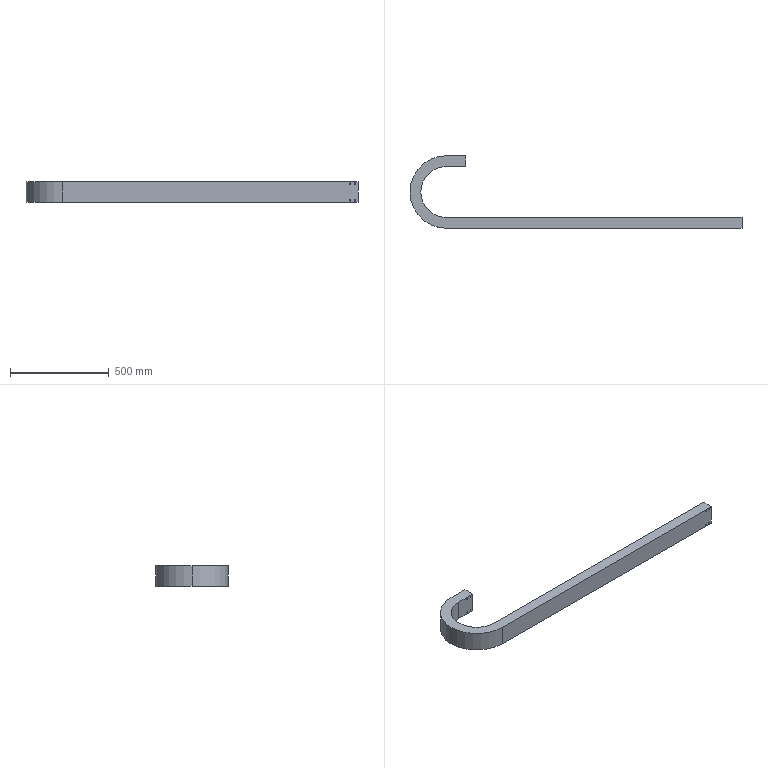Part | NX | features BREP 1 | 1 solid | 40 faces | box 1684 x 368 x 102 mm | volume 6232156 mm3 | cylinder 22 | plane 18 | commonest cylinder face diameters 5.5 x8 6 x8 258 x2 368 x2 278 x1 348 x1
STEP:
#1=CARTESIAN_POINT('',(1460.2,-184.,5.25));
#2=VERTEX_POINT('',#1);
#3=CARTESIAN_POINT('',(1460.2,-184.,11.25));
#4=VERTEX_POINT('',#3);
#5=CARTESIAN_POINT('',(1460.2,-184.,8.25));
#6=DIRECTION('',(0.,1.,0.));
#7=DIRECTION('',(0.,0.,1.));
#8=AXIS2_PLACEMENT_3D('',#5,#6,#7);
#9=CIRCLE('',#8,3.);
#10=EDGE_CURVE('',#2,#4,#9,.T.);
#11=ORIENTED_EDGE('',*,*,#10,.F.);
#12=CARTESIAN_POINT('',(1460.2,-129.,5.25));
#13=VERTEX_POINT('',#12);
#14=CARTESIAN_POINT('',(1460.2,-231.,5.25));
#15=DIRECTION('',(0.,1.,0.));
#16=VECTOR('',#15,1000.);
#17=LINE('',#14,#16);
#18=EDGE_CURVE('',#13,#2,#17,.F.);
#19=ORIENTED_EDGE('',*,*,#18,.F.);
#20=CARTESIAN_POINT('',(1460.2,-129.,11.25));
#21=VERTEX_POINT('',#20);
#22=CARTESIAN_POINT('',(1460.2,-129.,8.25));
#23=DIRECTION('',(0.,1.,0.));
#24=DIRECTION('',(0.,0.,1.));
#25=AXIS2_PLACEMENT_3D('',#22,#23,#24);
#26=CIRCLE('',#25,3.);
#27=EDGE_CURVE('',#13,#21,#26,.T.);
#28=ORIENTED_EDGE('',*,*,#27,.T.);
#29=CARTESIAN_POINT('',(1460.2,-231.,11.25));
#30=DIRECTION('',(0.,1.,0.));
#31=VECTOR('',#30,1000.);
#32=LINE('',#29,#31);
#33=EDGE_CURVE('',#21,#4,#32,.F.);
#34=ORIENTED_EDGE('',*,*,#33,.T.);
#35=EDGE_LOOP('',(#11,#19,#28,#34));
#36=FACE_BOUND('',#35,.T.);
#37=CARTESIAN_POINT('',(1460.2,-231.,8.25));
#38=DIRECTION('',(0.,1.,0.));
#39=DIRECTION('',(0.,0.,1.));
#40=AXIS2_PLACEMENT_3D('',#37,#38,#39);
#41=CYLINDRICAL_SURFACE('',#40,3.);
#42=ADVANCED_FACE('',(#36),#41,.F.);
#43=CARTESIAN_POINT('',(1484.35,-184.,90.75));
#44=VERTEX_POINT('',#43);
#45=CARTESIAN_POINT('',(1484.35,-184.,96.75));
#46=VERTEX_POINT('',#45);
#47=CARTESIAN_POINT('',(1484.35,-184.,93.75));
#48=DIRECTION('',(0.,1.,0.));
#49=DIRECTION('',(0.,0.,1.));
#50=AXIS2_PLACEMENT_3D('',#47,#48,#49);
#51=CIRCLE('',#50,3.);
#52=EDGE_CURVE('',#44,#46,#51,.T.);
#53=ORIENTED_EDGE('',*,*,#52,.F.);
#54=CARTESIAN_POINT('',(1484.35,-129.,90.75));
#55=VERTEX_POINT('',#54);
#56=CARTESIAN_POINT('',(1484.35,-231.,90.75));
#57=DIRECTION('',(0.,1.,0.));
#58=VECTOR('',#57,1000.);
#59=LINE('',#56,#58);
#60=EDGE_CURVE('',#55,#44,#59,.F.);
#61=ORIENTED_EDGE('',*,*,#60,.F.);
#62=CARTESIAN_POINT('',(1484.35,-129.,96.75));
#63=VERTEX_POINT('',#62);
#64=CARTESIAN_POINT('',(1484.35,-129.,93.75));
#65=DIRECTION('',(0.,1.,0.));
#66=DIRECTION('',(0.,0.,1.));
#67=AXIS2_PLACEMENT_3D('',#64,#65,#66);
#68=CIRCLE('',#67,3.);
#69=EDGE_CURVE('',#55,#63,#68,.T.);
#70=ORIENTED_EDGE('',*,*,#69,.T.);
#71=CARTESIAN_POINT('',(1484.35,-231.,96.75));
#72=DIRECTION('',(0.,1.,0.));
#73=VECTOR('',#72,1000.);
#74=LINE('',#71,#73);
#75=EDGE_CURVE('',#63,#46,#74,.F.);
#76=ORIENTED_EDGE('',*,*,#75,.T.);
#77=EDGE_LOOP('',(#53,#61,#70,#76));
#78=FACE_BOUND('',#77,.T.);
#79=CARTESIAN_POINT('',(1484.35,-231.,93.75));
#80=DIRECTION('',(0.,1.,0.));
#81=DIRECTION('',(0.,0.,1.));
#82=AXIS2_PLACEMENT_3D('',#79,#80,#81);
#83=CYLINDRICAL_SURFACE('',#82,3.);
#84=ADVANCED_FACE('',(#78),#83,.F.);
#85=CARTESIAN_POINT('',(1460.2,-184.,90.75));
#86=VERTEX_POINT('',#85);
#87=CARTESIAN_POINT('',(1460.2,-184.,96.75));
#88=VERTEX_POINT('',#87);
#89=CARTESIAN_POINT('',(1460.2,-184.,93.75));
#90=DIRECTION('',(0.,1.,0.));
#91=DIRECTION('',(0.,0.,1.));
#92=AXIS2_PLACEMENT_3D('',#89,#90,#91);
#93=CIRCLE('',#92,3.);
#94=EDGE_CURVE('',#86,#88,#93,.T.);
#95=ORIENTED_EDGE('',*,*,#94,.F.);
#96=CARTESIAN_POINT('',(1460.2,-129.,90.75));
#97=VERTEX_POINT('',#96);
#98=CARTESIAN_POINT('',(1460.2,-231.,90.75));
#99=DIRECTION('',(0.,1.,0.));
#100=VECTOR('',#99,1000.);
#101=LINE('',#98,#100);
#102=EDGE_CURVE('',#97,#86,#101,.F.);
#103=ORIENTED_EDGE('',*,*,#102,.F.);
#104=CARTESIAN_POINT('',(1460.2,-129.,96.75));
#105=VERTEX_POINT('',#104);
#106=CARTESIAN_POINT('',(1460.2,-129.,93.75));
#107=DIRECTION('',(0.,1.,0.));
#108=DIRECTION('',(0.,0.,1.));
#109=AXIS2_PLACEMENT_3D('',#106,#107,#108);
#110=CIRCLE('',#109,3.);
#111=EDGE_CURVE('',#97,#105,#110,.T.);
#112=ORIENTED_EDGE('',*,*,#111,.T.);
#113=CARTESIAN_POINT('',(1460.2,-231.,96.75));
#114=DIRECTION('',(0.,1.,0.));
#115=VECTOR('',#114,1000.);
#116=LINE('',#113,#115);
#117=EDGE_CURVE('',#105,#88,#116,.F.);
#118=ORIENTED_EDGE('',*,*,#117,.T.);
#119=EDGE_LOOP('',(#95,#103,#112,#118));
#120=FACE_BOUND('',#119,.T.);
#121=CARTESIAN_POINT('',(1460.2,-231.,93.75));
#122=DIRECTION('',(0.,1.,0.));
#123=DIRECTION('',(0.,0.,1.));
#124=AXIS2_PLACEMENT_3D('',#121,#122,#123);
#125=CYLINDRICAL_SURFACE('',#124,3.);
#126=ADVANCED_FACE('',(#120),#125,.F.);
#127=CARTESIAN_POINT('',(1484.35,-184.,5.25));
#128=VERTEX_POINT('',#127);
#129=CARTESIAN_POINT('',(1484.35,-184.,11.25));
#130=VERTEX_POINT('',#129);
#131=CARTESIAN_POINT('',(1484.35,-184.,8.25));
#132=DIRECTION('',(0.,1.,0.));
#133=DIRECTION('',(0.,0.,1.));
#134=AXIS2_PLACEMENT_3D('',#131,#132,#133);
#135=CIRCLE('',#134,3.);
#136=EDGE_CURVE('',#128,#130,#135,.T.);
#137=ORIENTED_EDGE('',*,*,#136,.F.);
#138=CARTESIAN_POINT('',(1484.35,-129.,5.25));
#139=VERTEX_POINT('',#138);
#140=CARTESIAN_POINT('',(1484.35,-231.,5.25));
#141=DIRECTION('',(0.,1.,0.));
#142=VECTOR('',#141,1000.);
#143=LINE('',#140,#142);
#144=EDGE_CURVE('',#139,#128,#143,.F.);
#145=ORIENTED_EDGE('',*,*,#144,.F.);
#146=CARTESIAN_POINT('',(1484.35,-129.,11.25));
#147=VERTEX_POINT('',#146);
#148=CARTESIAN_POINT('',(1484.35,-129.,8.25));
#149=DIRECTION('',(0.,1.,0.));
#150=DIRECTION('',(0.,0.,1.));
#151=AXIS2_PLACEMENT_3D('',#148,#149,#150);
#152=CIRCLE('',#151,3.);
#153=EDGE_CURVE('',#139,#147,#152,.T.);
#154=ORIENTED_EDGE('',*,*,#153,.T.);
#155=CARTESIAN_POINT('',(1484.35,-231.,11.25));
#156=DIRECTION('',(0.,1.,0.));
#157=VECTOR('',#156,1000.);
#158=LINE('',#155,#157);
#159=EDGE_CURVE('',#147,#130,#158,.F.);
#160=ORIENTED_EDGE('',*,*,#159,.T.);
#161=EDGE_LOOP('',(#137,#145,#154,#160));
#162=FACE_BOUND('',#161,.T.);
#163=CARTESIAN_POINT('',(1484.35,-231.,8.25));
#164=DIRECTION('',(0.,1.,0.));
#165=DIRECTION('',(0.,0.,1.));
#166=AXIS2_PLACEMENT_3D('',#163,#164,#165);
#167=CYLINDRICAL_SURFACE('',#166,3.);
#168=ADVANCED_FACE('',(#162),#167,.F.);
#169=CARTESIAN_POINT('',(84.35,129.,5.5));
#170=VERTEX_POINT('',#169);
#171=CARTESIAN_POINT('',(84.35,129.,11.));
#172=VERTEX_POINT('',#171);
#173=CARTESIAN_POINT('',(84.35,129.,8.25));
#174=DIRECTION('',(0.,1.,0.));
#175=DIRECTION('',(0.,0.,1.));
#176=AXIS2_PLACEMENT_3D('',#173,#174,#175);
#177=CIRCLE('',#176,2.75);
#178=EDGE_CURVE('',#170,#172,#177,.T.);
#179=ORIENTED_EDGE('',*,*,#178,.F.);
#180=CARTESIAN_POINT('',(84.35,184.,5.5));
#181=VERTEX_POINT('',#180);
#182=CARTESIAN_POINT('',(84.35,184.,5.5));
#183=DIRECTION('',(0.,1.,0.));
#184=VECTOR('',#183,1000.);
#185=LINE('',#182,#184);
#186=EDGE_CURVE('',#181,#170,#185,.F.);
#187=ORIENTED_EDGE('',*,*,#186,.F.);
#188=CARTESIAN_POINT('',(84.35,184.,11.));
#189=VERTEX_POINT('',#188);
#190=CARTESIAN_POINT('',(84.35,184.,8.25));
#191=DIRECTION('',(0.,1.,0.));
#192=DIRECTION('',(0.,0.,1.));
#193=AXIS2_PLACEMENT_3D('',#190,#191,#192);
#194=CIRCLE('',#193,2.75);
#195=EDGE_CURVE('',#181,#189,#194,.T.);
#196=ORIENTED_EDGE('',*,*,#195,.T.);
#197=CARTESIAN_POINT('',(84.35,184.,11.));
#198=DIRECTION('',(0.,1.,0.));
#199=VECTOR('',#198,1000.);
#200=LINE('',#197,#199);
#201=EDGE_CURVE('',#189,#172,#200,.F.);
#202=ORIENTED_EDGE('',*,*,#201,.T.);
#203=EDGE_LOOP('',(#179,#187,#196,#202));
#204=FACE_BOUND('',#203,.T.);
#205=CARTESIAN_POINT('',(84.35,184.,8.25));
#206=DIRECTION('',(0.,1.,0.));
#207=DIRECTION('',(0.,0.,1.));
#208=AXIS2_PLACEMENT_3D('',#205,#206,#207);
#209=CYLINDRICAL_SURFACE('',#208,2.75);
#210=ADVANCED_FACE('',(#204),#209,.F.);
#211=CARTESIAN_POINT('',(60.2,129.,5.5));
#212=VERTEX_POINT('',#211);
#213=CARTESIAN_POINT('',(60.2,129.,11.));
#214=VERTEX_POINT('',#213);
#215=CARTESIAN_POINT('',(60.2,129.,8.25));
#216=DIRECTION('',(0.,1.,0.));
#217=DIRECTION('',(0.,0.,1.));
#218=AXIS2_PLACEMENT_3D('',#215,#216,#217);
#219=CIRCLE('',#218,2.75);
#220=EDGE_CURVE('',#212,#214,#219,.T.);
#221=ORIENTED_EDGE('',*,*,#220,.F.);
#222=CARTESIAN_POINT('',(60.2,184.,5.5));
#223=VERTEX_POINT('',#222);
#224=CARTESIAN_POINT('',(60.2,184.,5.5));
#225=DIRECTION('',(0.,1.,0.));
#226=VECTOR('',#225,1000.);
#227=LINE('',#224,#226);
#228=EDGE_CURVE('',#223,#212,#227,.F.);
#229=ORIENTED_EDGE('',*,*,#228,.F.);
#230=CARTESIAN_POINT('',(60.2,184.,11.));
#231=VERTEX_POINT('',#230);
#232=CARTESIAN_POINT('',(60.2,184.,8.25));
#233=DIRECTION('',(0.,1.,0.));
#234=DIRECTION('',(0.,0.,1.));
#235=AXIS2_PLACEMENT_3D('',#232,#233,#234);
#236=CIRCLE('',#235,2.75);
#237=EDGE_CURVE('',#223,#231,#236,.T.);
#238=ORIENTED_EDGE('',*,*,#237,.T.);
#239=CARTESIAN_POINT('',(60.2,184.,11.));
#240=DIRECTION('',(0.,1.,0.));
#241=VECTOR('',#240,1000.);
#242=LINE('',#239,#241);
#243=EDGE_CURVE('',#231,#214,#242,.F.);
#244=ORIENTED_EDGE('',*,*,#243,.T.);
#245=EDGE_LOOP('',(#221,#229,#238,#244));
#246=FACE_BOUND('',#245,.T.);
#247=CARTESIAN_POINT('',(60.2,184.,8.25));
#248=DIRECTION('',(0.,1.,0.));
#249=DIRECTION('',(0.,0.,1.));
#250=AXIS2_PLACEMENT_3D('',#247,#248,#249);
#251=CYLINDRICAL_SURFACE('',#250,2.75);
#252=ADVANCED_FACE('',(#246),#251,.F.);
#253=CARTESIAN_POINT('',(60.2,129.,91.));
#254=VERTEX_POINT('',#253);
#255=CARTESIAN_POINT('',(60.2,129.,96.5));
#256=VERTEX_POINT('',#255);
#257=CARTESIAN_POINT('',(60.2,129.,93.75));
#258=DIRECTION('',(0.,1.,0.));
#259=DIRECTION('',(0.,0.,1.));
#260=AXIS2_PLACEMENT_3D('',#257,#258,#259);
#261=CIRCLE('',#260,2.75);
#262=EDGE_CURVE('',#254,#256,#261,.T.);
#263=ORIENTED_EDGE('',*,*,#262,.F.);
#264=CARTESIAN_POINT('',(60.2,184.,91.));
#265=VERTEX_POINT('',#264);
#266=CARTESIAN_POINT('',(60.2,184.,91.));
#267=DIRECTION('',(0.,1.,0.));
#268=VECTOR('',#267,1000.);
#269=LINE('',#266,#268);
#270=EDGE_CURVE('',#265,#254,#269,.F.);
#271=ORIENTED_EDGE('',*,*,#270,.F.);
#272=CARTESIAN_POINT('',(60.2,184.,96.5));
#273=VERTEX_POINT('',#272);
#274=CARTESIAN_POINT('',(60.2,184.,93.75));
#275=DIRECTION('',(0.,1.,0.));
#276=DIRECTION('',(0.,0.,1.));
#277=AXIS2_PLACEMENT_3D('',#274,#275,#276);
#278=CIRCLE('',#277,2.75);
#279=EDGE_CURVE('',#265,#273,#278,.T.);
#280=ORIENTED_EDGE('',*,*,#279,.T.);
#281=CARTESIAN_POINT('',(60.2,184.,96.5));
#282=DIRECTION('',(0.,1.,0.));
#283=VECTOR('',#282,1000.);
#284=LINE('',#281,#283);
#285=EDGE_CURVE('',#273,#256,#284,.F.);
#286=ORIENTED_EDGE('',*,*,#285,.T.);
#287=EDGE_LOOP('',(#263,#271,#280,#286));
#288=FACE_BOUND('',#287,.T.);
#289=CARTESIAN_POINT('',(60.2,184.,93.75));
#290=DIRECTION('',(0.,1.,0.));
#291=DIRECTION('',(0.,0.,1.));
#292=AXIS2_PLACEMENT_3D('',#289,#290,#291);
#293=CYLINDRICAL_SURFACE('',#292,2.75);
#294=ADVANCED_FACE('',(#288),#293,.F.);
#295=CARTESIAN_POINT('',(84.35,129.,91.));
#296=VERTEX_POINT('',#295);
#297=CARTESIAN_POINT('',(84.35,129.,96.5));
#298=VERTEX_POINT('',#297);
#299=CARTESIAN_POINT('',(84.35,129.,93.75));
#300=DIRECTION('',(0.,1.,0.));
#301=DIRECTION('',(0.,0.,1.));
#302=AXIS2_PLACEMENT_3D('',#299,#300,#301);
#303=CIRCLE('',#302,2.75);
#304=EDGE_CURVE('',#296,#298,#303,.T.);
#305=ORIENTED_EDGE('',*,*,#304,.F.);
#306=CARTESIAN_POINT('',(84.35,184.,91.));
#307=VERTEX_POINT('',#306);
#308=CARTESIAN_POINT('',(84.35,184.,91.));
#309=DIRECTION('',(0.,1.,0.));
#310=VECTOR('',#309,1000.);
#311=LINE('',#308,#310);
#312=EDGE_CURVE('',#307,#296,#311,.F.);
#313=ORIENTED_EDGE('',*,*,#312,.F.);
#314=CARTESIAN_POINT('',(84.35,184.,96.5));
#315=VERTEX_POINT('',#314);
#316=CARTESIAN_POINT('',(84.35,184.,93.75));
#317=DIRECTION('',(0.,1.,0.));
#318=DIRECTION('',(0.,0.,1.));
#319=AXIS2_PLACEMENT_3D('',#316,#317,#318);
#320=CIRCLE('',#319,2.75);
#321=EDGE_CURVE('',#307,#315,#320,.T.);
#322=ORIENTED_EDGE('',*,*,#321,.T.);
#323=CARTESIAN_POINT('',(84.35,184.,96.5));
#324=DIRECTION('',(0.,1.,0.));
#325=VECTOR('',#324,1000.);
#326=LINE('',#323,#325);
#327=EDGE_CURVE('',#315,#298,#326,.F.);
#328=ORIENTED_EDGE('',*,*,#327,.T.);
#329=EDGE_LOOP('',(#305,#313,#322,#328));
#330=FACE_BOUND('',#329,.T.);
#331=CARTESIAN_POINT('',(84.35,184.,93.75));
#332=DIRECTION('',(0.,1.,0.));
#333=DIRECTION('',(0.,0.,1.));
#334=AXIS2_PLACEMENT_3D('',#331,#332,#333);
#335=CYLINDRICAL_SURFACE('',#334,2.75);
#336=ADVANCED_FACE('',(#330),#335,.F.);
#337=CARTESIAN_POINT('',(-184.,0.,102.));
#338=VERTEX_POINT('',#337);
#339=CARTESIAN_POINT('',(0.,-184.,102.));
#340=VERTEX_POINT('',#339);
#341=CARTESIAN_POINT('',(0.,0.,102.));
#342=DIRECTION('',(0.,0.,1.));
#343=DIRECTION('',(1.,0.,0.));
#344=AXIS2_PLACEMENT_3D('',#341,#342,#343);
#345=CIRCLE('',#344,184.);
#346=EDGE_CURVE('',#338,#340,#345,.T.);
#347=ORIENTED_EDGE('',*,*,#346,.F.);
#348=CARTESIAN_POINT('',(-184.,0.,0.));
#349=VERTEX_POINT('',#348);
#350=CARTESIAN_POINT('',(-184.,0.,102.));
#351=DIRECTION('',(0.,0.,-1.));
#352=VECTOR('',#351,1000.);
#353=LINE('',#350,#352);
#354=EDGE_CURVE('',#338,#349,#353,.T.);
#355=ORIENTED_EDGE('',*,*,#354,.T.);
#356=CARTESIAN_POINT('',(0.,-184.,0.));
#357=VERTEX_POINT('',#356);
#358=CARTESIAN_POINT('',(0.,0.,0.));
#359=DIRECTION('',(0.,0.,1.));
#360=DIRECTION('',(1.,0.,0.));
#361=AXIS2_PLACEMENT_3D('',#358,#359,#360);
#362=CIRCLE('',#361,184.);
#363=EDGE_CURVE('',#349,#357,#362,.T.);
#364=ORIENTED_EDGE('',*,*,#363,.T.);
#365=CARTESIAN_POINT('',(0.,-184.,102.));
#366=DIRECTION('',(0.,0.,-1.));
#367=VECTOR('',#366,1000.);
#368=LINE('',#365,#367);
#369=EDGE_CURVE('',#340,#357,#368,.T.);
#370=ORIENTED_EDGE('',*,*,#369,.F.);
#371=EDGE_LOOP('',(#347,#355,#364,#370));
#372=FACE_BOUND('',#371,.T.);
#373=CARTESIAN_POINT('',(0.,0.,102.));
#374=DIRECTION('',(0.,0.,-1.));
#375=DIRECTION('',(-1.,0.,0.));
#376=AXIS2_PLACEMENT_3D('',#373,#374,#375);
#377=CYLINDRICAL_SURFACE('',#376,184.);
#378=ADVANCED_FACE('',(#372),#377,.T.);
#379=CARTESIAN_POINT('',(-129.,0.,102.));
#380=VERTEX_POINT('',#379);
#381=CARTESIAN_POINT('',(0.,129.,102.));
#382=VERTEX_POINT('',#381);
#383=CARTESIAN_POINT('',(0.,0.,102.));
#384=DIRECTION('',(0.,0.,-1.));
#385=DIRECTION('',(1.,0.,0.));
#386=AXIS2_PLACEMENT_3D('',#383,#384,#385);
#387=CIRCLE('',#386,129.);
#388=EDGE_CURVE('',#380,#382,#387,.T.);
#389=ORIENTED_EDGE('',*,*,#388,.F.);
#390=CARTESIAN_POINT('',(-129.,0.,0.));
#391=VERTEX_POINT('',#390);
#392=CARTESIAN_POINT('',(-129.,0.,102.));
#393=DIRECTION('',(0.,0.,-1.));
#394=VECTOR('',#393,1000.);
#395=LINE('',#392,#394);
#396=EDGE_CURVE('',#380,#391,#395,.T.);
#397=ORIENTED_EDGE('',*,*,#396,.T.);
#398=CARTESIAN_POINT('',(0.,129.,0.));
#399=VERTEX_POINT('',#398);
#400=CARTESIAN_POINT('',(0.,0.,0.));
#401=DIRECTION('',(0.,0.,-1.));
#402=DIRECTION('',(1.,0.,0.));
#403=AXIS2_PLACEMENT_3D('',#400,#401,#402);
#404=CIRCLE('',#403,129.);
#405=EDGE_CURVE('',#391,#399,#404,.T.);
#406=ORIENTED_EDGE('',*,*,#405,.T.);
#407=CARTESIAN_POINT('',(0.,129.,102.));
#408=DIRECTION('',(0.,0.,-1.));
#409=VECTOR('',#408,1000.);
#410=LINE('',#407,#409);
#411=EDGE_CURVE('',#382,#399,#410,.T.);
#412=ORIENTED_EDGE('',*,*,#411,.F.);
#413=EDGE_LOOP('',(#389,#397,#406,#412));
#414=FACE_BOUND('',#413,.T.);
#415=CARTESIAN_POINT('',(0.,0.,102.));
#416=DIRECTION('',(0.,0.,-1.));
#417=DIRECTION('',(-1.,0.,0.));
#418=AXIS2_PLACEMENT_3D('',#415,#416,#417);
#419=CYLINDRICAL_SURFACE('',#418,129.);
#420=ADVANCED_FACE('',(#414),#419,.F.);
#421=CARTESIAN_POINT('',(100.,129.,0.));
#422=VERTEX_POINT('',#421);
#423=CARTESIAN_POINT('',(100.,184.,0.));
#424=VERTEX_POINT('',#423);
#425=CARTESIAN_POINT('',(100.,129.,0.));
#426=DIRECTION('',(0.,1.,0.));
#427=VECTOR('',#426,1000.);
#428=LINE('',#425,#427);
#429=EDGE_CURVE('',#422,#424,#428,.T.);
#430=ORIENTED_EDGE('',*,*,#429,.T.);
#431=CARTESIAN_POINT('',(100.,184.,102.));
#432=VERTEX_POINT('',#431);
#433=CARTESIAN_POINT('',(100.,184.,102.));
#434=DIRECTION('',(0.,0.,-1.));
#435=VECTOR('',#434,1000.);
#436=LINE('',#433,#435);
#437=EDGE_CURVE('',#432,#424,#436,.T.);
#438=ORIENTED_EDGE('',*,*,#437,.F.);
#439=CARTESIAN_POINT('',(100.,129.,102.));
#440=VERTEX_POINT('',#439);
#441=CARTESIAN_POINT('',(100.,129.,102.));
#442=DIRECTION('',(0.,1.,0.));
#443=VECTOR('',#442,1000.);
#444=LINE('',#441,#443);
#445=EDGE_CURVE('',#440,#432,#444,.T.);
#446=ORIENTED_EDGE('',*,*,#445,.F.);
#447=CARTESIAN_POINT('',(100.,129.,102.));
#448=DIRECTION('',(0.,0.,-1.));
#449=VECTOR('',#448,1000.);
#450=LINE('',#447,#449);
#451=EDGE_CURVE('',#440,#422,#450,.T.);
#452=ORIENTED_EDGE('',*,*,#451,.T.);
#453=EDGE_LOOP('',(#430,#438,#446,#452));
#454=FACE_BOUND('',#453,.T.);
#455=CARTESIAN_POINT('',(100.,139.,88.5));
#456=VERTEX_POINT('',#455);
#457=CARTESIAN_POINT('',(100.,174.,88.5));
#458=VERTEX_POINT('',#457);
#459=CARTESIAN_POINT('',(100.,174.,88.5));
#460=DIRECTION('',(0.,1.,0.));
#461=VECTOR('',#460,1000.);
#462=LINE('',#459,#461);
#463=EDGE_CURVE('',#456,#458,#462,.T.);
#464=ORIENTED_EDGE('',*,*,#463,.T.);
#465=CARTESIAN_POINT('',(100.,174.,13.5));
#466=VERTEX_POINT('',#465);
#467=CARTESIAN_POINT('',(100.,174.,88.5));
#468=DIRECTION('',(0.,0.,-1.));
#469=VECTOR('',#468,1000.);
#470=LINE('',#467,#469);
#471=EDGE_CURVE('',#458,#466,#470,.T.);
#472=ORIENTED_EDGE('',*,*,#471,.T.);
#473=CARTESIAN_POINT('',(100.,139.,13.5));
#474=VERTEX_POINT('',#473);
#475=CARTESIAN_POINT('',(100.,174.,13.5));
#476=DIRECTION('',(0.,-1.,0.));
#477=VECTOR('',#476,1000.);
#478=LINE('',#475,#477);
#479=EDGE_CURVE('',#466,#474,#478,.T.);
#480=ORIENTED_EDGE('',*,*,#479,.T.);
#481=CARTESIAN_POINT('',(100.,139.,88.5));
#482=DIRECTION('',(0.,0.,1.));
#483=VECTOR('',#482,1000.);
#484=LINE('',#481,#483);
#485=EDGE_CURVE('',#474,#456,#484,.T.);
#486=ORIENTED_EDGE('',*,*,#485,.T.);
#487=EDGE_LOOP('',(#464,#472,#480,#486));
#488=FACE_BOUND('',#487,.T.);
#489=CARTESIAN_POINT('',(100.,129.,102.));
#490=DIRECTION('',(-1.,0.,0.));
#491=DIRECTION('',(0.,0.,1.));
#492=AXIS2_PLACEMENT_3D('',#489,#490,#491);
#493=PLANE('',#492);
#494=ADVANCED_FACE('',(#454,#488),#493,.F.);
#495=CARTESIAN_POINT('',(1500.,-184.,0.));
#496=VERTEX_POINT('',#495);
#497=CARTESIAN_POINT('',(1500.,-129.,0.));
#498=VERTEX_POINT('',#497);
#499=CARTESIAN_POINT('',(1500.,-184.,0.));
#500=DIRECTION('',(0.,1.,0.));
#501=VECTOR('',#500,1000.);
#502=LINE('',#499,#501);
#503=EDGE_CURVE('',#496,#498,#502,.T.);
#504=ORIENTED_EDGE('',*,*,#503,.T.);
#505=CARTESIAN_POINT('',(1500.,-129.,102.));
#506=VERTEX_POINT('',#505);
#507=CARTESIAN_POINT('',(1500.,-129.,102.));
#508=DIRECTION('',(0.,0.,-1.));
#509=VECTOR('',#508,1000.);
#510=LINE('',#507,#509);
#511=EDGE_CURVE('',#506,#498,#510,.T.);
#512=ORIENTED_EDGE('',*,*,#511,.F.);
#513=CARTESIAN_POINT('',(1500.,-184.,102.));
#514=VERTEX_POINT('',#513);
#515=CARTESIAN_POINT('',(1500.,-184.,102.));
#516=DIRECTION('',(0.,1.,0.));
#517=VECTOR('',#516,1000.);
#518=LINE('',#515,#517);
#519=EDGE_CURVE('',#514,#506,#518,.T.);
#520=ORIENTED_EDGE('',*,*,#519,.F.);
#521=CARTESIAN_POINT('',(1500.,-184.,102.));
#522=DIRECTION('',(0.,0.,-1.));
#523=VECTOR('',#522,1000.);
#524=LINE('',#521,#523);
#525=EDGE_CURVE('',#514,#496,#524,.T.);
#526=ORIENTED_EDGE('',*,*,#525,.T.);
#527=EDGE_LOOP('',(#504,#512,#520,#526));
#528=FACE_BOUND('',#527,.T.);
#529=CARTESIAN_POINT('',(1500.,-174.,88.5));
#530=VERTEX_POINT('',#529);
#531=CARTESIAN_POINT('',(1500.,-139.,88.5));
#532=VERTEX_POINT('',#531);
#533=CARTESIAN_POINT('',(1500.,-174.,88.5));
#534=DIRECTION('',(0.,1.,0.));
#535=VECTOR('',#534,1000.);
#536=LINE('',#533,#535);
#537=EDGE_CURVE('',#530,#532,#536,.T.);
#538=ORIENTED_EDGE('',*,*,#537,.T.);
#539=CARTESIAN_POINT('',(1500.,-139.,13.5));
#540=VERTEX_POINT('',#539);
#541=CARTESIAN_POINT('',(1500.,-139.,88.5));
#542=DIRECTION('',(0.,0.,-1.));
#543=VECTOR('',#542,1000.);
#544=LINE('',#541,#543);
#545=EDGE_CURVE('',#532,#540,#544,.T.);
#546=ORIENTED_EDGE('',*,*,#545,.T.);
#547=CARTESIAN_POINT('',(1500.,-174.,13.5));
#548=VERTEX_POINT('',#547);
#549=CARTESIAN_POINT('',(1500.,-174.,13.5));
#550=DIRECTION('',(0.,-1.,0.));
#551=VECTOR('',#550,1000.);
#552=LINE('',#549,#551);
#553=EDGE_CURVE('',#540,#548,#552,.T.);
#554=ORIENTED_EDGE('',*,*,#553,.T.);
#555=CARTESIAN_POINT('',(1500.,-174.,88.5));
#556=DIRECTION('',(0.,0.,1.));
#557=VECTOR('',#556,1000.);
#558=LINE('',#555,#557);
#559=EDGE_CURVE('',#548,#530,#558,.T.);
#560=ORIENTED_EDGE('',*,*,#559,.T.);
#561=EDGE_LOOP('',(#538,#546,#554,#560));
#562=FACE_BOUND('',#561,.T.);
#563=CARTESIAN_POINT('',(1500.,-184.,102.));
#564=DIRECTION('',(-1.,0.,0.));
#565=DIRECTION('',(0.,0.,1.));
#566=AXIS2_PLACEMENT_3D('',#563,#564,#565);
#567=PLANE('',#566);
#568=ADVANCED_FACE('',(#528,#562),#567,.F.);
#569=ORIENTED_EDGE('',*,*,#396,.F.);
#570=CARTESIAN_POINT('',(0.,-129.,102.));
#571=VERTEX_POINT('',#570);
#572=CARTESIAN_POINT('',(0.,0.,102.));
#573=DIRECTION('',(0.,0.,-1.));
#574=DIRECTION('',(1.,0.,0.));
#575=AXIS2_PLACEMENT_3D('',#572,#573,#574);
#576=CIRCLE('',#575,129.);
#577=EDGE_CURVE('',#571,#380,#576,.T.);
#578=ORIENTED_EDGE('',*,*,#577,.F.);
#579=CARTESIAN_POINT('',(0.,-129.,0.));
#580=VERTEX_POINT('',#579);
#581=CARTESIAN_POINT('',(0.,-129.,102.));
#582=DIRECTION('',(0.,0.,-1.));
#583=VECTOR('',#582,1000.);
#584=LINE('',#581,#583);
#585=EDGE_CURVE('',#571,#580,#584,.T.);
#586=ORIENTED_EDGE('',*,*,#585,.T.);
#587=CARTESIAN_POINT('',(0.,0.,0.));
#588=DIRECTION('',(0.,0.,-1.));
#589=DIRECTION('',(1.,0.,0.));
#590=AXIS2_PLACEMENT_3D('',#587,#588,#589);
#591=CIRCLE('',#590,129.);
#592=EDGE_CURVE('',#580,#391,#591,.T.);
#593=ORIENTED_EDGE('',*,*,#592,.T.);
#594=EDGE_LOOP('',(#569,#578,#586,#593));
#595=FACE_BOUND('',#594,.T.);
#596=CARTESIAN_POINT('',(0.,0.,102.));
#597=DIRECTION('',(0.,0.,-1.));
#598=DIRECTION('',(-1.,0.,0.));
#599=AXIS2_PLACEMENT_3D('',#596,#597,#598);
#600=CYLINDRICAL_SURFACE('',#599,129.);
#601=ADVANCED_FACE('',(#595),#600,.F.);
#602=CARTESIAN_POINT('',(0.,129.,0.));
#603=DIRECTION('',(1.,0.,0.));
#604=VECTOR('',#603,1000.);
#605=LINE('',#602,#604);
#606=EDGE_CURVE('',#399,#422,#605,.T.);
#607=ORIENTED_EDGE('',*,*,#606,.T.);
#608=ORIENTED_EDGE('',*,*,#451,.F.);
#609=CARTESIAN_POINT('',(0.,129.,102.));
#610=DIRECTION('',(1.,0.,0.));
#611=VECTOR('',#610,1000.);
#612=LINE('',#609,#611);
#613=EDGE_CURVE('',#382,#440,#612,.T.);
#614=ORIENTED_EDGE('',*,*,#613,.F.);
#615=ORIENTED_EDGE('',*,*,#411,.T.);
#616=EDGE_LOOP('',(#607,#608,#614,#615));
#617=FACE_BOUND('',#616,.T.);
#618=CARTESIAN_POINT('',(84.35,129.,8.25));
#619=DIRECTION('',(0.,1.,0.));
#620=DIRECTION('',(0.,0.,1.));
#621=AXIS2_PLACEMENT_3D('',#618,#619,#620);
#622=CIRCLE('',#621,2.75);
#623=EDGE_CURVE('',#172,#170,#622,.T.);
#624=ORIENTED_EDGE('',*,*,#623,.T.);
#625=ORIENTED_EDGE('',*,*,#178,.T.);
#626=EDGE_LOOP('',(#624,#625));
#627=FACE_BOUND('',#626,.T.);
#628=CARTESIAN_POINT('',(60.2,129.,8.25));
#629=DIRECTION('',(0.,1.,0.));
#630=DIRECTION('',(0.,0.,1.));
#631=AXIS2_PLACEMENT_3D('',#628,#629,#630);
#632=CIRCLE('',#631,2.75);
#633=EDGE_CURVE('',#214,#212,#632,.T.);
#634=ORIENTED_EDGE('',*,*,#633,.T.);
#635=ORIENTED_EDGE('',*,*,#220,.T.);
#636=EDGE_LOOP('',(#634,#635));
#637=FACE_BOUND('',#636,.T.);
#638=CARTESIAN_POINT('',(60.2,129.,93.75));
#639=DIRECTION('',(0.,1.,0.));
#640=DIRECTION('',(0.,0.,1.));
#641=AXIS2_PLACEMENT_3D('',#638,#639,#640);
#642=CIRCLE('',#641,2.75);
#643=EDGE_CURVE('',#256,#254,#642,.T.);
#644=ORIENTED_EDGE('',*,*,#643,.T.);
#645=ORIENTED_EDGE('',*,*,#262,.T.);
#646=EDGE_LOOP('',(#644,#645));
#647=FACE_BOUND('',#646,.T.);
#648=CARTESIAN_POINT('',(84.35,129.,93.75));
#649=DIRECTION('',(0.,1.,0.));
#650=DIRECTION('',(0.,0.,1.));
#651=AXIS2_PLACEMENT_3D('',#648,#649,#650);
#652=CIRCLE('',#651,2.75);
#653=EDGE_CURVE('',#298,#296,#652,.T.);
#654=ORIENTED_EDGE('',*,*,#653,.T.);
#655=ORIENTED_EDGE('',*,*,#304,.T.);
#656=EDGE_LOOP('',(#654,#655));
#657=FACE_BOUND('',#656,.T.);
#658=CARTESIAN_POINT('',(0.,129.,102.));
#659=DIRECTION('',(0.,1.,0.));
#660=DIRECTION('',(1.,0.,0.));
#661=AXIS2_PLACEMENT_3D('',#658,#659,#660);
#662=PLANE('',#661);
#663=ADVANCED_FACE('',(#617,#627,#637,#647,#657),#662,.F.);
#664=CARTESIAN_POINT('',(0.,184.,0.));
#665=VERTEX_POINT('',#664);
#666=CARTESIAN_POINT('',(100.,184.,0.));
#667=DIRECTION('',(-1.,0.,0.));
#668=VECTOR('',#667,1000.);
#669=LINE('',#666,#668);
#670=EDGE_CURVE('',#424,#665,#669,.T.);
#671=ORIENTED_EDGE('',*,*,#670,.T.);
#672=CARTESIAN_POINT('',(0.,184.,102.));
#673=VERTEX_POINT('',#672);
#674=CARTESIAN_POINT('',(0.,184.,102.));
#675=DIRECTION('',(0.,0.,-1.));
#676=VECTOR('',#675,1000.);
#677=LINE('',#674,#676);
#678=EDGE_CURVE('',#673,#665,#677,.T.);
#679=ORIENTED_EDGE('',*,*,#678,.F.);
#680=CARTESIAN_POINT('',(100.,184.,102.));
#681=DIRECTION('',(-1.,0.,0.));
#682=VECTOR('',#681,1000.);
#683=LINE('',#680,#682);
#684=EDGE_CURVE('',#432,#673,#683,.T.);
#685=ORIENTED_EDGE('',*,*,#684,.F.);
#686=ORIENTED_EDGE('',*,*,#437,.T.);
#687=EDGE_LOOP('',(#671,#679,#685,#686));
#688=FACE_BOUND('',#687,.T.);
#689=CARTESIAN_POINT('',(84.35,184.,8.25));
#690=DIRECTION('',(0.,1.,0.));
#691=DIRECTION('',(0.,0.,1.));
#692=AXIS2_PLACEMENT_3D('',#689,#690,#691);
#693=CIRCLE('',#692,2.75);
#694=EDGE_CURVE('',#189,#181,#693,.T.);
#695=ORIENTED_EDGE('',*,*,#694,.F.);
#696=ORIENTED_EDGE('',*,*,#195,.F.);
#697=EDGE_LOOP('',(#695,#696));
#698=FACE_BOUND('',#697,.T.);
#699=CARTESIAN_POINT('',(60.2,184.,8.25));
#700=DIRECTION('',(0.,1.,0.));
#701=DIRECTION('',(0.,0.,1.));
#702=AXIS2_PLACEMENT_3D('',#699,#700,#701);
#703=CIRCLE('',#702,2.75);
#704=EDGE_CURVE('',#231,#223,#703,.T.);
#705=ORIENTED_EDGE('',*,*,#704,.F.);
#706=ORIENTED_EDGE('',*,*,#237,.F.);
#707=EDGE_LOOP('',(#705,#706));
#708=FACE_BOUND('',#707,.T.);
#709=CARTESIAN_POINT('',(60.2,184.,93.75));
#710=DIRECTION('',(0.,1.,0.));
#711=DIRECTION('',(0.,0.,1.));
#712=AXIS2_PLACEMENT_3D('',#709,#710,#711);
#713=CIRCLE('',#712,2.75);
#714=EDGE_CURVE('',#273,#265,#713,.T.);
#715=ORIENTED_EDGE('',*,*,#714,.F.);
#716=ORIENTED_EDGE('',*,*,#279,.F.);
#717=EDGE_LOOP('',(#715,#716));
#718=FACE_BOUND('',#717,.T.);
#719=CARTESIAN_POINT('',(84.35,184.,93.75));
#720=DIRECTION('',(0.,1.,0.));
#721=DIRECTION('',(0.,0.,1.));
#722=AXIS2_PLACEMENT_3D('',#719,#720,#721);
#723=CIRCLE('',#722,2.75);
#724=EDGE_CURVE('',#315,#307,#723,.T.);
#725=ORIENTED_EDGE('',*,*,#724,.F.);
#726=ORIENTED_EDGE('',*,*,#321,.F.);
#727=EDGE_LOOP('',(#725,#726));
#728=FACE_BOUND('',#727,.T.);
#729=CARTESIAN_POINT('',(100.,184.,102.));
#730=DIRECTION('',(0.,-1.,0.));
#731=DIRECTION('',(-1.,0.,0.));
#732=AXIS2_PLACEMENT_3D('',#729,#730,#731);
#733=PLANE('',#732);
#734=ADVANCED_FACE('',(#688,#698,#708,#718,#728),#733,.F.);
#735=ORIENTED_EDGE('',*,*,#354,.F.);
#736=CARTESIAN_POINT('',(0.,0.,102.));
#737=DIRECTION('',(0.,0.,1.));
#738=DIRECTION('',(1.,0.,0.));
#739=AXIS2_PLACEMENT_3D('',#736,#737,#738);
#740=CIRCLE('',#739,184.);
#741=EDGE_CURVE('',#673,#338,#740,.T.);
#742=ORIENTED_EDGE('',*,*,#741,.F.);
#743=ORIENTED_EDGE('',*,*,#678,.T.);
#744=CARTESIAN_POINT('',(0.,0.,0.));
#745=DIRECTION('',(0.,0.,1.));
#746=DIRECTION('',(1.,0.,0.));
#747=AXIS2_PLACEMENT_3D('',#744,#745,#746);
#748=CIRCLE('',#747,184.);
#749=EDGE_CURVE('',#665,#349,#748,.T.);
#750=ORIENTED_EDGE('',*,*,#749,.T.);
#751=EDGE_LOOP('',(#735,#742,#743,#750));
#752=FACE_BOUND('',#751,.T.);
#753=CARTESIAN_POINT('',(0.,0.,102.));
#754=DIRECTION('',(0.,0.,-1.));
#755=DIRECTION('',(-1.,0.,0.));
#756=AXIS2_PLACEMENT_3D('',#753,#754,#755);
#757=CYLINDRICAL_SURFACE('',#756,184.);
#758=ADVANCED_FACE('',(#752),#757,.T.);
#759=CARTESIAN_POINT('',(0.,-184.,0.));
#760=DIRECTION('',(1.,0.,0.));
#761=VECTOR('',#760,1000.);
#762=LINE('',#759,#761);
#763=EDGE_CURVE('',#357,#496,#762,.T.);
#764=ORIENTED_EDGE('',*,*,#763,.T.);
#765=ORIENTED_EDGE('',*,*,#525,.F.);
#766=CARTESIAN_POINT('',(0.,-184.,102.));
#767=DIRECTION('',(1.,0.,0.));
#768=VECTOR('',#767,1000.);
#769=LINE('',#766,#768);
#770=EDGE_CURVE('',#340,#514,#769,.T.);
#771=ORIENTED_EDGE('',*,*,#770,.F.);
#772=ORIENTED_EDGE('',*,*,#369,.T.);
#773=EDGE_LOOP('',(#764,#765,#771,#772));
#774=FACE_BOUND('',#773,.T.);
#775=CARTESIAN_POINT('',(1460.2,-184.,8.25));
#776=DIRECTION('',(0.,1.,0.));
#777=DIRECTION('',(0.,0.,1.));
#778=AXIS2_PLACEMENT_3D('',#775,#776,#777);
#779=CIRCLE('',#778,3.);
#780=EDGE_CURVE('',#4,#2,#779,.T.);
#781=ORIENTED_EDGE('',*,*,#780,.T.);
#782=ORIENTED_EDGE('',*,*,#10,.T.);
#783=EDGE_LOOP('',(#781,#782));
#784=FACE_BOUND('',#783,.T.);
#785=CARTESIAN_POINT('',(1484.35,-184.,93.75));
#786=DIRECTION('',(0.,1.,0.));
#787=DIRECTION('',(0.,0.,1.));
#788=AXIS2_PLACEMENT_3D('',#785,#786,#787);
#789=CIRCLE('',#788,3.);
#790=EDGE_CURVE('',#46,#44,#789,.T.);
#791=ORIENTED_EDGE('',*,*,#790,.T.);
#792=ORIENTED_EDGE('',*,*,#52,.T.);
#793=EDGE_LOOP('',(#791,#792));
#794=FACE_BOUND('',#793,.T.);
#795=CARTESIAN_POINT('',(1460.2,-184.,93.75));
#796=DIRECTION('',(0.,1.,0.));
#797=DIRECTION('',(0.,0.,1.));
#798=AXIS2_PLACEMENT_3D('',#795,#796,#797);
#799=CIRCLE('',#798,3.);
#800=EDGE_CURVE('',#88,#86,#799,.T.);
#801=ORIENTED_EDGE('',*,*,#800,.T.);
#802=ORIENTED_EDGE('',*,*,#94,.T.);
#803=EDGE_LOOP('',(#801,#802));
#804=FACE_BOUND('',#803,.T.);
#805=CARTESIAN_POINT('',(1484.35,-184.,8.25));
#806=DIRECTION('',(0.,1.,0.));
#807=DIRECTION('',(0.,0.,1.));
#808=AXIS2_PLACEMENT_3D('',#805,#806,#807);
#809=CIRCLE('',#808,3.);
#810=EDGE_CURVE('',#130,#128,#809,.T.);
#811=ORIENTED_EDGE('',*,*,#810,.T.);
#812=ORIENTED_EDGE('',*,*,#136,.T.);
#813=EDGE_LOOP('',(#811,#812));
#814=FACE_BOUND('',#813,.T.);
#815=CARTESIAN_POINT('',(0.,-184.,102.));
#816=DIRECTION('',(0.,1.,0.));
#817=DIRECTION('',(1.,0.,0.));
#818=AXIS2_PLACEMENT_3D('',#815,#816,#817);
#819=PLANE('',#818);
#820=ADVANCED_FACE('',(#774,#784,#794,#804,#814),#819,.F.);
#821=CARTESIAN_POINT('',(0.,-129.,0.));
#822=DIRECTION('',(-1.,0.,0.));
#823=VECTOR('',#822,1000.);
#824=LINE('',#821,#823);
#825=EDGE_CURVE('',#498,#580,#824,.T.);
#826=ORIENTED_EDGE('',*,*,#825,.T.);
#827=ORIENTED_EDGE('',*,*,#585,.F.);
#828=CARTESIAN_POINT('',(0.,-129.,102.));
#829=DIRECTION('',(-1.,0.,0.));
#830=VECTOR('',#829,1000.);
#831=LINE('',#828,#830);
#832=EDGE_CURVE('',#506,#571,#831,.T.);
#833=ORIENTED_EDGE('',*,*,#832,.F.);
#834=ORIENTED_EDGE('',*,*,#511,.T.);
#835=EDGE_LOOP('',(#826,#827,#833,#834));
#836=FACE_BOUND('',#835,.T.);
#837=CARTESIAN_POINT('',(1460.2,-129.,8.25));
#838=DIRECTION('',(0.,1.,0.));
#839=DIRECTION('',(0.,0.,1.));
#840=AXIS2_PLACEMENT_3D('',#837,#838,#839);
#841=CIRCLE('',#840,3.);
#842=EDGE_CURVE('',#21,#13,#841,.T.);
#843=ORIENTED_EDGE('',*,*,#842,.F.);
#844=ORIENTED_EDGE('',*,*,#27,.F.);
#845=EDGE_LOOP('',(#843,#844));
#846=FACE_BOUND('',#845,.T.);
#847=CARTESIAN_POINT('',(1484.35,-129.,93.75));
#848=DIRECTION('',(0.,1.,0.));
#849=DIRECTION('',(0.,0.,1.));
#850=AXIS2_PLACEMENT_3D('',#847,#848,#849);
#851=CIRCLE('',#850,3.);
#852=EDGE_CURVE('',#63,#55,#851,.T.);
#853=ORIENTED_EDGE('',*,*,#852,.F.);
#854=ORIENTED_EDGE('',*,*,#69,.F.);
#855=EDGE_LOOP('',(#853,#854));
#856=FACE_BOUND('',#855,.T.);
#857=CARTESIAN_POINT('',(1460.2,-129.,93.75));
#858=DIRECTION('',(0.,1.,0.));
#859=DIRECTION('',(0.,0.,1.));
#860=AXIS2_PLACEMENT_3D('',#857,#858,#859);
#861=CIRCLE('',#860,3.);
#862=EDGE_CURVE('',#105,#97,#861,.T.);
#863=ORIENTED_EDGE('',*,*,#862,.F.);
#864=ORIENTED_EDGE('',*,*,#111,.F.);
#865=EDGE_LOOP('',(#863,#864));
#866=FACE_BOUND('',#865,.T.);
#867=CARTESIAN_POINT('',(1484.35,-129.,8.25));
#868=DIRECTION('',(0.,1.,0.));
#869=DIRECTION('',(0.,0.,1.));
#870=AXIS2_PLACEMENT_3D('',#867,#868,#869);
#871=CIRCLE('',#870,3.);
#872=EDGE_CURVE('',#147,#139,#871,.T.);
#873=ORIENTED_EDGE('',*,*,#872,.F.);
#874=ORIENTED_EDGE('',*,*,#153,.F.);
#875=EDGE_LOOP('',(#873,#874));
#876=FACE_BOUND('',#875,.T.);
#877=CARTESIAN_POINT('',(0.,-129.,102.));
#878=DIRECTION('',(0.,-1.,0.));
#879=DIRECTION('',(0.,0.,-1.));
#880=AXIS2_PLACEMENT_3D('',#877,#878,#879);
#881=PLANE('',#880);
#882=ADVANCED_FACE('',(#836,#846,#856,#866,#876),#881,.F.);
#883=ORIENTED_EDGE('',*,*,#577,.T.);
#884=ORIENTED_EDGE('',*,*,#388,.T.);
#885=ORIENTED_EDGE('',*,*,#613,.T.);
#886=ORIENTED_EDGE('',*,*,#445,.T.);
#887=ORIENTED_EDGE('',*,*,#684,.T.);
#888=ORIENTED_EDGE('',*,*,#741,.T.);
#889=ORIENTED_EDGE('',*,*,#346,.T.);
#890=ORIENTED_EDGE('',*,*,#770,.T.);
#891=ORIENTED_EDGE('',*,*,#519,.T.);
#892=ORIENTED_EDGE('',*,*,#832,.T.);
#893=EDGE_LOOP('',(#883,#884,#885,#886,#887,#888,#889,#890,#891,#892));
#894=FACE_BOUND('',#893,.T.);
#895=CARTESIAN_POINT('',(0.,0.,102.));
#896=DIRECTION('',(0.,0.,1.));
#897=DIRECTION('',(1.,0.,0.));
#898=AXIS2_PLACEMENT_3D('',#895,#896,#897);
#899=PLANE('',#898);
#900=ADVANCED_FACE('',(#894),#899,.T.);
#901=ORIENTED_EDGE('',*,*,#592,.F.);
#902=ORIENTED_EDGE('',*,*,#825,.F.);
#903=ORIENTED_EDGE('',*,*,#503,.F.);
#904=ORIENTED_EDGE('',*,*,#763,.F.);
#905=ORIENTED_EDGE('',*,*,#363,.F.);
#906=ORIENTED_EDGE('',*,*,#749,.F.);
#907=ORIENTED_EDGE('',*,*,#670,.F.);
#908=ORIENTED_EDGE('',*,*,#429,.F.);
#909=ORIENTED_EDGE('',*,*,#606,.F.);
#910=ORIENTED_EDGE('',*,*,#405,.F.);
#911=EDGE_LOOP('',(#901,#902,#903,#904,#905,#906,#907,#908,#909,#910));
#912=FACE_BOUND('',#911,.T.);
#913=CARTESIAN_POINT('',(0.,0.,0.));
#914=DIRECTION('',(0.,0.,1.));
#915=DIRECTION('',(1.,0.,0.));
#916=AXIS2_PLACEMENT_3D('',#913,#914,#915);
#917=PLANE('',#916);
#918=ADVANCED_FACE('',(#912),#917,.F.);
#919=CARTESIAN_POINT('',(0.,-174.,13.5));
#920=VERTEX_POINT('',#919);
#921=CARTESIAN_POINT('',(0.,-174.,13.5));
#922=DIRECTION('',(1.,0.,0.));
#923=VECTOR('',#922,1000.);
#924=LINE('',#921,#923);
#925=EDGE_CURVE('',#920,#548,#924,.T.);
#926=ORIENTED_EDGE('',*,*,#925,.F.);
#927=CARTESIAN_POINT('',(0.,-174.,88.5));
#928=VERTEX_POINT('',#927);
#929=CARTESIAN_POINT('',(0.,-174.,88.5));
#930=DIRECTION('',(0.,0.,1.));
#931=VECTOR('',#930,1000.);
#932=LINE('',#929,#931);
#933=EDGE_CURVE('',#920,#928,#932,.T.);
#934=ORIENTED_EDGE('',*,*,#933,.T.);
#935=CARTESIAN_POINT('',(0.,-174.,88.5));
#936=DIRECTION('',(1.,0.,0.));
#937=VECTOR('',#936,1000.);
#938=LINE('',#935,#937);
#939=EDGE_CURVE('',#928,#530,#938,.T.);
#940=ORIENTED_EDGE('',*,*,#939,.T.);
#941=ORIENTED_EDGE('',*,*,#559,.F.);
#942=EDGE_LOOP('',(#926,#934,#940,#941));
#943=FACE_BOUND('',#942,.T.);
#944=CARTESIAN_POINT('',(0.,-174.,88.5));
#945=DIRECTION('',(0.,1.,0.));
#946=DIRECTION('',(1.,0.,0.));
#947=AXIS2_PLACEMENT_3D('',#944,#945,#946);
#948=PLANE('',#947);
#949=ADVANCED_FACE('',(#943),#948,.T.);
#950=CARTESIAN_POINT('',(0.,-139.,13.5));
#951=VERTEX_POINT('',#950);
#952=CARTESIAN_POINT('',(0.,-139.,13.5));
#953=DIRECTION('',(1.,0.,0.));
#954=VECTOR('',#953,1000.);
#955=LINE('',#952,#954);
#956=EDGE_CURVE('',#951,#540,#955,.T.);
#957=ORIENTED_EDGE('',*,*,#956,.F.);
#958=CARTESIAN_POINT('',(0.,-174.,13.5));
#959=DIRECTION('',(0.,-1.,0.));
#960=VECTOR('',#959,1000.);
#961=LINE('',#958,#960);
#962=EDGE_CURVE('',#951,#920,#961,.T.);
#963=ORIENTED_EDGE('',*,*,#962,.T.);
#964=ORIENTED_EDGE('',*,*,#925,.T.);
#965=ORIENTED_EDGE('',*,*,#553,.F.);
#966=EDGE_LOOP('',(#957,#963,#964,#965));
#967=FACE_BOUND('',#966,.T.);
#968=CARTESIAN_POINT('',(0.,-174.,13.5));
#969=DIRECTION('',(0.,0.,1.));
#970=DIRECTION('',(1.,0.,0.));
#971=AXIS2_PLACEMENT_3D('',#968,#969,#970);
#972=PLANE('',#971);
#973=ADVANCED_FACE('',(#967),#972,.T.);
#974=CARTESIAN_POINT('',(0.,-139.,88.5));
#975=VERTEX_POINT('',#974);
#976=CARTESIAN_POINT('',(0.,-139.,88.5));
#977=DIRECTION('',(1.,0.,0.));
#978=VECTOR('',#977,1000.);
#979=LINE('',#976,#978);
#980=EDGE_CURVE('',#975,#532,#979,.T.);
#981=ORIENTED_EDGE('',*,*,#980,.F.);
#982=CARTESIAN_POINT('',(0.,-139.,88.5));
#983=DIRECTION('',(0.,0.,-1.));
#984=VECTOR('',#983,1000.);
#985=LINE('',#982,#984);
#986=EDGE_CURVE('',#975,#951,#985,.T.);
#987=ORIENTED_EDGE('',*,*,#986,.T.);
#988=ORIENTED_EDGE('',*,*,#956,.T.);
#989=ORIENTED_EDGE('',*,*,#545,.F.);
#990=EDGE_LOOP('',(#981,#987,#988,#989));
#991=FACE_BOUND('',#990,.T.);
#992=CARTESIAN_POINT('',(0.,-139.,88.5));
#993=DIRECTION('',(0.,-1.,0.));
#994=DIRECTION('',(0.,0.,-1.));
#995=AXIS2_PLACEMENT_3D('',#992,#993,#994);
#996=PLANE('',#995);
#997=ADVANCED_FACE('',(#991),#996,.T.);
#998=ORIENTED_EDGE('',*,*,#939,.F.);
#999=CARTESIAN_POINT('',(0.,-174.,88.5));
#1000=DIRECTION('',(0.,1.,0.));
#1001=VECTOR('',#1000,1000.);
#1002=LINE('',#999,#1001);
#1003=EDGE_CURVE('',#928,#975,#1002,.T.);
#1004=ORIENTED_EDGE('',*,*,#1003,.T.);
#1005=ORIENTED_EDGE('',*,*,#980,.T.);
#1006=ORIENTED_EDGE('',*,*,#537,.F.);
#1007=EDGE_LOOP('',(#998,#1004,#1005,#1006));
#1008=FACE_BOUND('',#1007,.T.);
#1009=CARTESIAN_POINT('',(0.,-174.,88.5));
#1010=DIRECTION('',(0.,0.,-1.));
#1011=DIRECTION('',(0.,-1.,0.));
#1012=AXIS2_PLACEMENT_3D('',#1009,#1010,#1011);
#1013=PLANE('',#1012);
#1014=ADVANCED_FACE('',(#1008),#1013,.T.);
#1015=ORIENTED_EDGE('',*,*,#933,.F.);
#1016=CARTESIAN_POINT('',(0.,174.,13.5));
#1017=VERTEX_POINT('',#1016);
#1018=CARTESIAN_POINT('',(0.,0.,13.5));
#1019=DIRECTION('',(0.,0.,1.));
#1020=DIRECTION('',(0.,1.,0.));
#1021=AXIS2_PLACEMENT_3D('',#1018,#1019,#1020);
#1022=CIRCLE('',#1021,174.);
#1023=EDGE_CURVE('',#1017,#920,#1022,.T.);
#1024=ORIENTED_EDGE('',*,*,#1023,.F.);
#1025=CARTESIAN_POINT('',(0.,174.,88.5));
#1026=VERTEX_POINT('',#1025);
#1027=CARTESIAN_POINT('',(0.,174.,88.5));
#1028=DIRECTION('',(0.,0.,1.));
#1029=VECTOR('',#1028,1000.);
#1030=LINE('',#1027,#1029);
#1031=EDGE_CURVE('',#1017,#1026,#1030,.T.);
#1032=ORIENTED_EDGE('',*,*,#1031,.T.);
#1033=CARTESIAN_POINT('',(0.,0.,88.5));
#1034=DIRECTION('',(0.,0.,1.));
#1035=DIRECTION('',(0.,1.,0.));
#1036=AXIS2_PLACEMENT_3D('',#1033,#1034,#1035);
#1037=CIRCLE('',#1036,174.);
#1038=EDGE_CURVE('',#1026,#928,#1037,.T.);
#1039=ORIENTED_EDGE('',*,*,#1038,.T.);
#1040=EDGE_LOOP('',(#1015,#1024,#1032,#1039));
#1041=FACE_BOUND('',#1040,.T.);
#1042=CARTESIAN_POINT('',(0.,0.,102.));
#1043=DIRECTION('',(0.,0.,1.));
#1044=DIRECTION('',(1.,0.,0.));
#1045=AXIS2_PLACEMENT_3D('',#1042,#1043,#1044);
#1046=CYLINDRICAL_SURFACE('',#1045,174.);
#1047=ADVANCED_FACE('',(#1041),#1046,.F.);
#1048=ORIENTED_EDGE('',*,*,#1023,.T.);
#1049=ORIENTED_EDGE('',*,*,#962,.F.);
#1050=CARTESIAN_POINT('',(0.,139.,13.5));
#1051=VERTEX_POINT('',#1050);
#1052=CARTESIAN_POINT('',(0.,0.,13.5));
#1053=DIRECTION('',(0.,0.,1.));
#1054=DIRECTION('',(0.,1.,0.));
#1055=AXIS2_PLACEMENT_3D('',#1052,#1053,#1054);
#1056=CIRCLE('',#1055,139.);
#1057=EDGE_CURVE('',#1051,#951,#1056,.T.);
#1058=ORIENTED_EDGE('',*,*,#1057,.F.);
#1059=CARTESIAN_POINT('',(0.,174.,13.5));
#1060=DIRECTION('',(0.,1.,0.));
#1061=VECTOR('',#1060,1000.);
#1062=LINE('',#1059,#1061);
#1063=EDGE_CURVE('',#1051,#1017,#1062,.T.);
#1064=ORIENTED_EDGE('',*,*,#1063,.T.);
#1065=EDGE_LOOP('',(#1048,#1049,#1058,#1064));
#1066=FACE_BOUND('',#1065,.T.);
#1067=CARTESIAN_POINT('',(0.,174.,13.5));
#1068=DIRECTION('',(0.,0.,1.));
#1069=DIRECTION('',(1.,0.,0.));
#1070=AXIS2_PLACEMENT_3D('',#1067,#1068,#1069);
#1071=PLANE('',#1070);
#1072=ADVANCED_FACE('',(#1066),#1071,.T.);
#1073=ORIENTED_EDGE('',*,*,#1057,.T.);
#1074=ORIENTED_EDGE('',*,*,#986,.F.);
#1075=CARTESIAN_POINT('',(0.,139.,88.5));
#1076=VERTEX_POINT('',#1075);
#1077=CARTESIAN_POINT('',(0.,0.,88.5));
#1078=DIRECTION('',(0.,0.,1.));
#1079=DIRECTION('',(0.,1.,0.));
#1080=AXIS2_PLACEMENT_3D('',#1077,#1078,#1079);
#1081=CIRCLE('',#1080,139.);
#1082=EDGE_CURVE('',#1076,#975,#1081,.T.);
#1083=ORIENTED_EDGE('',*,*,#1082,.F.);
#1084=CARTESIAN_POINT('',(0.,139.,88.5));
#1085=DIRECTION('',(0.,0.,-1.));
#1086=VECTOR('',#1085,1000.);
#1087=LINE('',#1084,#1086);
#1088=EDGE_CURVE('',#1076,#1051,#1087,.T.);
#1089=ORIENTED_EDGE('',*,*,#1088,.T.);
#1090=EDGE_LOOP('',(#1073,#1074,#1083,#1089));
#1091=FACE_BOUND('',#1090,.T.);
#1092=CARTESIAN_POINT('',(0.,0.,102.));
#1093=DIRECTION('',(0.,0.,1.));
#1094=DIRECTION('',(1.,0.,0.));
#1095=AXIS2_PLACEMENT_3D('',#1092,#1093,#1094);
#1096=CYLINDRICAL_SURFACE('',#1095,139.);
#1097=ADVANCED_FACE('',(#1091),#1096,.T.);
#1098=ORIENTED_EDGE('',*,*,#1082,.T.);
#1099=ORIENTED_EDGE('',*,*,#1003,.F.);
#1100=ORIENTED_EDGE('',*,*,#1038,.F.);
#1101=CARTESIAN_POINT('',(0.,174.,88.5));
#1102=DIRECTION('',(0.,-1.,0.));
#1103=VECTOR('',#1102,1000.);
#1104=LINE('',#1101,#1103);
#1105=EDGE_CURVE('',#1026,#1076,#1104,.T.);
#1106=ORIENTED_EDGE('',*,*,#1105,.T.);
#1107=EDGE_LOOP('',(#1098,#1099,#1100,#1106));
#1108=FACE_BOUND('',#1107,.T.);
#1109=CARTESIAN_POINT('',(0.,174.,88.5));
#1110=DIRECTION('',(0.,0.,-1.));
#1111=DIRECTION('',(0.,-1.,0.));
#1112=AXIS2_PLACEMENT_3D('',#1109,#1110,#1111);
#1113=PLANE('',#1112);
#1114=ADVANCED_FACE('',(#1108),#1113,.T.);
#1115=CARTESIAN_POINT('',(104.,174.,88.5));
#1116=DIRECTION('',(-1.,0.,0.));
#1117=VECTOR('',#1116,1000.);
#1118=LINE('',#1115,#1117);
#1119=EDGE_CURVE('',#458,#1026,#1118,.T.);
#1120=ORIENTED_EDGE('',*,*,#1119,.T.);
#1121=ORIENTED_EDGE('',*,*,#1031,.F.);
#1122=CARTESIAN_POINT('',(104.,174.,13.5));
#1123=DIRECTION('',(-1.,0.,0.));
#1124=VECTOR('',#1123,1000.);
#1125=LINE('',#1122,#1124);
#1126=EDGE_CURVE('',#466,#1017,#1125,.T.);
#1127=ORIENTED_EDGE('',*,*,#1126,.F.);
#1128=ORIENTED_EDGE('',*,*,#471,.F.);
#1129=EDGE_LOOP('',(#1120,#1121,#1127,#1128));
#1130=FACE_BOUND('',#1129,.T.);
#1131=CARTESIAN_POINT('',(104.,174.,88.5));
#1132=DIRECTION('',(0.,-1.,0.));
#1133=DIRECTION('',(0.,0.,-1.));
#1134=AXIS2_PLACEMENT_3D('',#1131,#1132,#1133);
#1135=PLANE('',#1134);
#1136=ADVANCED_FACE('',(#1130),#1135,.T.);
#1137=ORIENTED_EDGE('',*,*,#1126,.T.);
#1138=ORIENTED_EDGE('',*,*,#1063,.F.);
#1139=CARTESIAN_POINT('',(104.,139.,13.5));
#1140=DIRECTION('',(-1.,0.,0.));
#1141=VECTOR('',#1140,1000.);
#1142=LINE('',#1139,#1141);
#1143=EDGE_CURVE('',#474,#1051,#1142,.T.);
#1144=ORIENTED_EDGE('',*,*,#1143,.F.);
#1145=ORIENTED_EDGE('',*,*,#479,.F.);
#1146=EDGE_LOOP('',(#1137,#1138,#1144,#1145));
#1147=FACE_BOUND('',#1146,.T.);
#1148=CARTESIAN_POINT('',(104.,174.,13.5));
#1149=DIRECTION('',(0.,0.,1.));
#1150=DIRECTION('',(1.,0.,0.));
#1151=AXIS2_PLACEMENT_3D('',#1148,#1149,#1150);
#1152=PLANE('',#1151);
#1153=ADVANCED_FACE('',(#1147),#1152,.T.);
#1154=ORIENTED_EDGE('',*,*,#1143,.T.);
#1155=ORIENTED_EDGE('',*,*,#1088,.F.);
#1156=CARTESIAN_POINT('',(104.,139.,88.5));
#1157=DIRECTION('',(-1.,0.,0.));
#1158=VECTOR('',#1157,1000.);
#1159=LINE('',#1156,#1158);
#1160=EDGE_CURVE('',#456,#1076,#1159,.T.);
#1161=ORIENTED_EDGE('',*,*,#1160,.F.);
#1162=ORIENTED_EDGE('',*,*,#485,.F.);
#1163=EDGE_LOOP('',(#1154,#1155,#1161,#1162));
#1164=FACE_BOUND('',#1163,.T.);
#1165=CARTESIAN_POINT('',(104.,139.,88.5));
#1166=DIRECTION('',(0.,1.,0.));
#1167=DIRECTION('',(1.,0.,0.));
#1168=AXIS2_PLACEMENT_3D('',#1165,#1166,#1167);
#1169=PLANE('',#1168);
#1170=ADVANCED_FACE('',(#1164),#1169,.T.);
#1171=ORIENTED_EDGE('',*,*,#1160,.T.);
#1172=ORIENTED_EDGE('',*,*,#1105,.F.);
#1173=ORIENTED_EDGE('',*,*,#1119,.F.);
#1174=ORIENTED_EDGE('',*,*,#463,.F.);
#1175=EDGE_LOOP('',(#1171,#1172,#1173,#1174));
#1176=FACE_BOUND('',#1175,.T.);
#1177=CARTESIAN_POINT('',(104.,174.,88.5));
#1178=DIRECTION('',(0.,0.,-1.));
#1179=DIRECTION('',(0.,-1.,0.));
#1180=AXIS2_PLACEMENT_3D('',#1177,#1178,#1179);
#1181=PLANE('',#1180);
#1182=ADVANCED_FACE('',(#1176),#1181,.T.);
#1183=ORIENTED_EDGE('',*,*,#312,.T.);
#1184=ORIENTED_EDGE('',*,*,#653,.F.);
#1185=ORIENTED_EDGE('',*,*,#327,.F.);
#1186=ORIENTED_EDGE('',*,*,#724,.T.);
#1187=EDGE_LOOP('',(#1183,#1184,#1185,#1186));
#1188=FACE_BOUND('',#1187,.T.);
#1189=CARTESIAN_POINT('',(84.35,184.,93.75));
#1190=DIRECTION('',(0.,1.,0.));
#1191=DIRECTION('',(0.,0.,1.));
#1192=AXIS2_PLACEMENT_3D('',#1189,#1190,#1191);
#1193=CYLINDRICAL_SURFACE('',#1192,2.75);
#1194=ADVANCED_FACE('',(#1188),#1193,.F.);
#1195=ORIENTED_EDGE('',*,*,#270,.T.);
#1196=ORIENTED_EDGE('',*,*,#643,.F.);
#1197=ORIENTED_EDGE('',*,*,#285,.F.);
#1198=ORIENTED_EDGE('',*,*,#714,.T.);
#1199=EDGE_LOOP('',(#1195,#1196,#1197,#1198));
#1200=FACE_BOUND('',#1199,.T.);
#1201=CARTESIAN_POINT('',(60.2,184.,93.75));
#1202=DIRECTION('',(0.,1.,0.));
#1203=DIRECTION('',(0.,0.,1.));
#1204=AXIS2_PLACEMENT_3D('',#1201,#1202,#1203);
#1205=CYLINDRICAL_SURFACE('',#1204,2.75);
#1206=ADVANCED_FACE('',(#1200),#1205,.F.);
#1207=ORIENTED_EDGE('',*,*,#228,.T.);
#1208=ORIENTED_EDGE('',*,*,#633,.F.);
#1209=ORIENTED_EDGE('',*,*,#243,.F.);
#1210=ORIENTED_EDGE('',*,*,#704,.T.);
#1211=EDGE_LOOP('',(#1207,#1208,#1209,#1210));
#1212=FACE_BOUND('',#1211,.T.);
#1213=CARTESIAN_POINT('',(60.2,184.,8.25));
#1214=DIRECTION('',(0.,1.,0.));
#1215=DIRECTION('',(0.,0.,1.));
#1216=AXIS2_PLACEMENT_3D('',#1213,#1214,#1215);
#1217=CYLINDRICAL_SURFACE('',#1216,2.75);
#1218=ADVANCED_FACE('',(#1212),#1217,.F.);
#1219=ORIENTED_EDGE('',*,*,#186,.T.);
#1220=ORIENTED_EDGE('',*,*,#623,.F.);
#1221=ORIENTED_EDGE('',*,*,#201,.F.);
#1222=ORIENTED_EDGE('',*,*,#694,.T.);
#1223=EDGE_LOOP('',(#1219,#1220,#1221,#1222));
#1224=FACE_BOUND('',#1223,.T.);
#1225=CARTESIAN_POINT('',(84.35,184.,8.25));
#1226=DIRECTION('',(0.,1.,0.));
#1227=DIRECTION('',(0.,0.,1.));
#1228=AXIS2_PLACEMENT_3D('',#1225,#1226,#1227);
#1229=CYLINDRICAL_SURFACE('',#1228,2.75);
#1230=ADVANCED_FACE('',(#1224),#1229,.F.);
#1231=ORIENTED_EDGE('',*,*,#144,.T.);
#1232=ORIENTED_EDGE('',*,*,#810,.F.);
#1233=ORIENTED_EDGE('',*,*,#159,.F.);
#1234=ORIENTED_EDGE('',*,*,#872,.T.);
#1235=EDGE_LOOP('',(#1231,#1232,#1233,#1234));
#1236=FACE_BOUND('',#1235,.T.);
#1237=CARTESIAN_POINT('',(1484.35,-231.,8.25));
#1238=DIRECTION('',(0.,1.,0.));
#1239=DIRECTION('',(0.,0.,1.));
#1240=AXIS2_PLACEMENT_3D('',#1237,#1238,#1239);
#1241=CYLINDRICAL_SURFACE('',#1240,3.);
#1242=ADVANCED_FACE('',(#1236),#1241,.F.);
#1243=ORIENTED_EDGE('',*,*,#102,.T.);
#1244=ORIENTED_EDGE('',*,*,#800,.F.);
#1245=ORIENTED_EDGE('',*,*,#117,.F.);
#1246=ORIENTED_EDGE('',*,*,#862,.T.);
#1247=EDGE_LOOP('',(#1243,#1244,#1245,#1246));
#1248=FACE_BOUND('',#1247,.T.);
#1249=CARTESIAN_POINT('',(1460.2,-231.,93.75));
#1250=DIRECTION('',(0.,1.,0.));
#1251=DIRECTION('',(0.,0.,1.));
#1252=AXIS2_PLACEMENT_3D('',#1249,#1250,#1251);
#1253=CYLINDRICAL_SURFACE('',#1252,3.);
#1254=ADVANCED_FACE('',(#1248),#1253,.F.);
#1255=ORIENTED_EDGE('',*,*,#60,.T.);
#1256=ORIENTED_EDGE('',*,*,#790,.F.);
#1257=ORIENTED_EDGE('',*,*,#75,.F.);
#1258=ORIENTED_EDGE('',*,*,#852,.T.);
#1259=EDGE_LOOP('',(#1255,#1256,#1257,#1258));
#1260=FACE_BOUND('',#1259,.T.);
#1261=CARTESIAN_POINT('',(1484.35,-231.,93.75));
#1262=DIRECTION('',(0.,1.,0.));
#1263=DIRECTION('',(0.,0.,1.));
#1264=AXIS2_PLACEMENT_3D('',#1261,#1262,#1263);
#1265=CYLINDRICAL_SURFACE('',#1264,3.);
#1266=ADVANCED_FACE('',(#1260),#1265,.F.);
#1267=ORIENTED_EDGE('',*,*,#18,.T.);
#1268=ORIENTED_EDGE('',*,*,#780,.F.);
#1269=ORIENTED_EDGE('',*,*,#33,.F.);
#1270=ORIENTED_EDGE('',*,*,#842,.T.);
#1271=EDGE_LOOP('',(#1267,#1268,#1269,#1270));
#1272=FACE_BOUND('',#1271,.T.);
#1273=CARTESIAN_POINT('',(1460.2,-231.,8.25));
#1274=DIRECTION('',(0.,1.,0.));
#1275=DIRECTION('',(0.,0.,1.));
#1276=AXIS2_PLACEMENT_3D('',#1273,#1274,#1275);
#1277=CYLINDRICAL_SURFACE('',#1276,3.);
#1278=ADVANCED_FACE('',(#1272),#1277,.F.);
#1279=CLOSED_SHELL('',(#42,#84,#126,#168,#210,#252,#294,#336,#378,#420,#494,#568,#601,#663,#734,#758,#820,#882,#900,#918,#949,#973,#997,#1014,#1047,#1072,#1097,#1114,#1136,#1153,#1170,#1182,#1194,#1206,#1218,#1230,#1242,#1254,#1266,#1278));
#1280=MANIFOLD_SOLID_BREP('',#1279);
#1281=(LENGTH_UNIT()NAMED_UNIT(*)SI_UNIT(.MILLI.,.METRE.));
#1282=UNCERTAINTY_MEASURE_WITH_UNIT(LENGTH_MEASURE(0.00001),#1281,'','');
#1283=(NAMED_UNIT(*)PLANE_ANGLE_UNIT()SI_UNIT($,.RADIAN.));
#1284=(NAMED_UNIT(*)SI_UNIT($,.STERADIAN.)SOLID_ANGLE_UNIT());
#1285=(GEOMETRIC_REPRESENTATION_CONTEXT(3)GLOBAL_UNCERTAINTY_ASSIGNED_CONTEXT((#1282))GLOBAL_UNIT_ASSIGNED_CONTEXT((#1281,#1283,#1284))REPRESENTATION_CONTEXT('',''));
#1286=ADVANCED_BREP_SHAPE_REPRESENTATION('',(#1280),#1285);